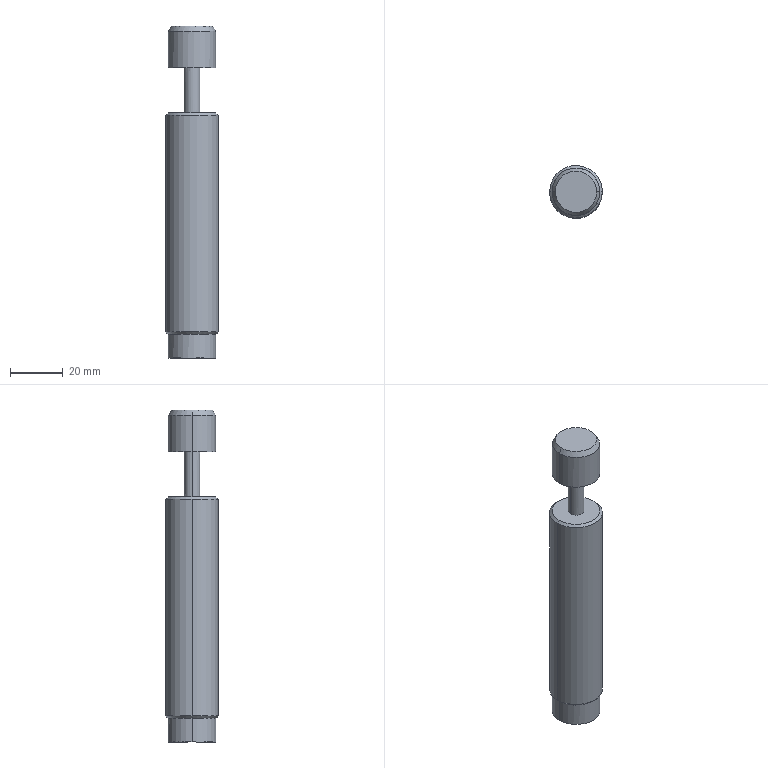Part | SolidWorks | features MoveFace 2, BaseBody 1 | 1 solid | 18 faces | box 20 x 20 x 126 mm | volume 33113 mm3 | cylinder 8 | cone 6 | plane 4 | commonest cylinder face diameters 6 x2 18 x2 18.16 x2 20 x2
STEP:
#1=CARTESIAN_POINT('',(-9.08,0.,-84.));
#2=VERTEX_POINT('',#1);
#3=CARTESIAN_POINT('',(9.08,0.,-84.));
#4=VERTEX_POINT('',#3);
#5=CARTESIAN_POINT('',(-9.08,0.,-84.));
#6=CARTESIAN_POINT('',(-9.08,1.189,-84.));
#7=CARTESIAN_POINT('',(-8.844,2.377,-84.));
#8=CARTESIAN_POINT('',(-7.934,4.573,-84.));
#9=CARTESIAN_POINT('',(-7.261,5.58,-84.));
#10=CARTESIAN_POINT('',(-5.58,7.261,-84.));
#11=CARTESIAN_POINT('',(-4.573,7.934,-84.));
#12=CARTESIAN_POINT('',(-2.377,8.844,-84.));
#13=CARTESIAN_POINT('',(-1.189,9.08,-84.));
#14=CARTESIAN_POINT('',(1.189,9.08,-84.));
#15=CARTESIAN_POINT('',(2.377,8.844,-84.));
#16=CARTESIAN_POINT('',(4.573,7.934,-84.));
#17=CARTESIAN_POINT('',(5.58,7.261,-84.));
#18=CARTESIAN_POINT('',(7.261,5.58,-84.));
#19=CARTESIAN_POINT('',(7.934,4.573,-84.));
#20=CARTESIAN_POINT('',(8.844,2.377,-84.));
#21=CARTESIAN_POINT('',(9.08,1.189,-84.));
#22=CARTESIAN_POINT('',(9.08,0.,-84.));
#23=B_SPLINE_CURVE_WITH_KNOTS('',3,(#5,#6,#7,#8,#9,#10,#11,#12,#13,#14,#15,#16,#17,#18,#19,#20,#21,#22),.UNSPECIFIED.,.F.,.F.,(4,2,2,2,2,2,2,2,4),(0.,0.3927,0.7854,1.178,1.571,1.963,2.356,2.749,3.142),.UNSPECIFIED.);
#24=EDGE_CURVE('',#2,#4,#23,.T.);
#25=ORIENTED_EDGE('',*,*,#24,.T.);
#26=CARTESIAN_POINT('',(9.08,0.,-93.));
#27=VERTEX_POINT('',#26);
#28=CARTESIAN_POINT('',(9.08,0.,-426.));
#29=DIRECTION('',(0.,0.,-1.));
#30=VECTOR('',#29,1000.);
#31=LINE('',#28,#30);
#32=EDGE_CURVE('',#4,#27,#31,.T.);
#33=ORIENTED_EDGE('',*,*,#32,.T.);
#34=CARTESIAN_POINT('',(-9.08,0.,-93.));
#35=VERTEX_POINT('',#34);
#36=CARTESIAN_POINT('',(-9.08,0.,-93.));
#37=CARTESIAN_POINT('',(-9.08,0.5962,-93.));
#38=CARTESIAN_POINT('',(-9.022,1.187,-93.));
#39=CARTESIAN_POINT('',(-8.789,2.356,-93.));
#40=CARTESIAN_POINT('',(-8.617,2.924,-93.));
#41=CARTESIAN_POINT('',(-8.161,4.026,-93.));
#42=CARTESIAN_POINT('',(-7.881,4.549,-93.));
#43=CARTESIAN_POINT('',(-7.219,5.54,-93.));
#44=CARTESIAN_POINT('',(-6.842,5.999,-93.));
#45=CARTESIAN_POINT('',(-5.999,6.842,-93.));
#46=CARTESIAN_POINT('',(-5.54,7.219,-93.));
#47=CARTESIAN_POINT('',(-4.549,7.881,-93.));
#48=CARTESIAN_POINT('',(-4.026,8.161,-93.));
#49=CARTESIAN_POINT('',(-2.924,8.617,-93.));
#50=CARTESIAN_POINT('',(-2.356,8.789,-93.));
#51=CARTESIAN_POINT('',(-1.187,9.022,-93.));
#52=CARTESIAN_POINT('',(-0.5962,9.08,-93.));
#53=CARTESIAN_POINT('',(0.5962,9.08,-93.));
#54=CARTESIAN_POINT('',(1.187,9.022,-93.));
#55=CARTESIAN_POINT('',(2.356,8.789,-93.));
#56=CARTESIAN_POINT('',(2.924,8.617,-93.));
#57=CARTESIAN_POINT('',(4.026,8.161,-93.));
#58=CARTESIAN_POINT('',(4.549,7.881,-93.));
#59=CARTESIAN_POINT('',(5.54,7.219,-93.));
#60=CARTESIAN_POINT('',(5.999,6.842,-93.));
#61=CARTESIAN_POINT('',(6.842,5.999,-93.));
#62=CARTESIAN_POINT('',(7.219,5.54,-93.));
#63=CARTESIAN_POINT('',(7.881,4.549,-93.));
#64=CARTESIAN_POINT('',(8.161,4.026,-93.));
#65=CARTESIAN_POINT('',(8.617,2.924,-93.));
#66=CARTESIAN_POINT('',(8.789,2.356,-93.));
#67=CARTESIAN_POINT('',(9.022,1.187,-93.));
#68=CARTESIAN_POINT('',(9.08,0.5962,-93.));
#69=CARTESIAN_POINT('',(9.08,0.,-93.));
#70=B_SPLINE_CURVE_WITH_KNOTS('',3,(#36,#37,#38,#39,#40,#41,#42,#43,#44,#45,#46,#47,#48,#49,#50,#51,#52,#53,#54,#55,#56,#57,#58,#59,#60,#61,#62,#63,#64,#65,#66,#67,#68,#69),.UNSPECIFIED.,.F.,.F.,(4,2,2,2,2,2,2,2,2,2,2,2,2,2,2,2,4),(0.,0.1963,0.3927,0.589,0.7854,0.9817,1.178,1.374,1.571,1.767,1.963,2.16,2.356,2.553,2.749,2.945,3.142),.UNSPECIFIED.);
#71=EDGE_CURVE('',#35,#27,#70,.T.);
#72=ORIENTED_EDGE('',*,*,#71,.F.);
#73=CARTESIAN_POINT('',(-9.08,0.,-426.));
#74=DIRECTION('',(0.,0.,-1.));
#75=VECTOR('',#74,1000.);
#76=LINE('',#73,#75);
#77=EDGE_CURVE('',#2,#35,#76,.T.);
#78=ORIENTED_EDGE('',*,*,#77,.F.);
#79=EDGE_LOOP('',(#25,#33,#72,#78));
#80=FACE_OUTER_BOUND('',#79,.T.);
#81=CARTESIAN_POINT('',(0.,0.,-426.));
#82=DIRECTION('',(0.,0.,-1.));
#83=DIRECTION('',(-1.,0.,0.));
#84=AXIS2_PLACEMENT_3D('',#81,#82,#83);
#85=CYLINDRICAL_SURFACE('',#84,9.08);
#86=ADVANCED_FACE('',(#80),#85,.T.);
#87=ORIENTED_EDGE('',*,*,#24,.F.);
#88=CARTESIAN_POINT('',(-10.,0.,-83.08));
#89=VERTEX_POINT('',#88);
#90=CARTESIAN_POINT('',(-10.,0.,-83.08));
#91=DIRECTION('',(-0.7071,0.,0.7071));
#92=VECTOR('',#91,1000.);
#93=LINE('',#90,#92);
#94=EDGE_CURVE('',#2,#89,#93,.T.);
#95=ORIENTED_EDGE('',*,*,#94,.T.);
#96=CARTESIAN_POINT('',(10.,0.,-83.08));
#97=VERTEX_POINT('',#96);
#98=CARTESIAN_POINT('',(-10.,0.,-83.08));
#99=CARTESIAN_POINT('',(-10.,1.309,-83.08));
#100=CARTESIAN_POINT('',(-9.74,2.617,-83.08));
#101=CARTESIAN_POINT('',(-8.738,5.036,-83.08));
#102=CARTESIAN_POINT('',(-7.997,6.145,-83.08));
#103=CARTESIAN_POINT('',(-6.145,7.997,-83.08));
#104=CARTESIAN_POINT('',(-5.036,8.738,-83.08));
#105=CARTESIAN_POINT('',(-2.617,9.74,-83.08));
#106=CARTESIAN_POINT('',(-1.309,10.,-83.08));
#107=CARTESIAN_POINT('',(1.309,10.,-83.08));
#108=CARTESIAN_POINT('',(2.617,9.74,-83.08));
#109=CARTESIAN_POINT('',(5.036,8.738,-83.08));
#110=CARTESIAN_POINT('',(6.145,7.997,-83.08));
#111=CARTESIAN_POINT('',(7.997,6.145,-83.08));
#112=CARTESIAN_POINT('',(8.738,5.036,-83.08));
#113=CARTESIAN_POINT('',(9.74,2.617,-83.08));
#114=CARTESIAN_POINT('',(10.,1.309,-83.08));
#115=CARTESIAN_POINT('',(10.,0.,-83.08));
#116=B_SPLINE_CURVE_WITH_KNOTS('',3,(#98,#99,#100,#101,#102,#103,#104,#105,#106,#107,#108,#109,#110,#111,#112,#113,#114,#115),.UNSPECIFIED.,.F.,.F.,(4,2,2,2,2,2,2,2,4),(0.,0.0625,0.125,0.1875,0.25,0.3125,0.375,0.4375,0.5),.UNSPECIFIED.);
#117=EDGE_CURVE('',#89,#97,#116,.T.);
#118=ORIENTED_EDGE('',*,*,#117,.T.);
#119=CARTESIAN_POINT('',(10.,0.,-83.08));
#120=DIRECTION('',(0.7071,0.,0.7071));
#121=VECTOR('',#120,1000.);
#122=LINE('',#119,#121);
#123=EDGE_CURVE('',#4,#97,#122,.T.);
#124=ORIENTED_EDGE('',*,*,#123,.F.);
#125=EDGE_LOOP('',(#87,#95,#118,#124));
#126=FACE_OUTER_BOUND('',#125,.T.);
#127=CARTESIAN_POINT('',(0.,0.,-83.08));
#128=DIRECTION('',(0.,0.,1.));
#129=DIRECTION('',(1.,0.,0.));
#130=AXIS2_PLACEMENT_3D('',#127,#128,#129);
#131=CONICAL_SURFACE('',#130,10.,0.7854);
#132=ADVANCED_FACE('',(#126),#131,.T.);
#133=CARTESIAN_POINT('',(-10.,0.,-0.92));
#134=VERTEX_POINT('',#133);
#135=CARTESIAN_POINT('',(10.,0.,-0.92));
#136=VERTEX_POINT('',#135);
#137=CARTESIAN_POINT('',(-10.,0.,-0.92));
#138=CARTESIAN_POINT('',(-10.,1.309,-0.92));
#139=CARTESIAN_POINT('',(-9.74,2.617,-0.92));
#140=CARTESIAN_POINT('',(-8.738,5.036,-0.92));
#141=CARTESIAN_POINT('',(-7.997,6.145,-0.92));
#142=CARTESIAN_POINT('',(-6.145,7.997,-0.92));
#143=CARTESIAN_POINT('',(-5.036,8.738,-0.92));
#144=CARTESIAN_POINT('',(-2.617,9.74,-0.92));
#145=CARTESIAN_POINT('',(-1.309,10.,-0.92));
#146=CARTESIAN_POINT('',(1.309,10.,-0.92));
#147=CARTESIAN_POINT('',(2.617,9.74,-0.92));
#148=CARTESIAN_POINT('',(5.036,8.738,-0.92));
#149=CARTESIAN_POINT('',(6.145,7.997,-0.92));
#150=CARTESIAN_POINT('',(7.997,6.145,-0.92));
#151=CARTESIAN_POINT('',(8.738,5.036,-0.92));
#152=CARTESIAN_POINT('',(9.74,2.617,-0.92));
#153=CARTESIAN_POINT('',(10.,1.309,-0.92));
#154=CARTESIAN_POINT('',(10.,0.,-0.92));
#155=B_SPLINE_CURVE_WITH_KNOTS('',3,(#137,#138,#139,#140,#141,#142,#143,#144,#145,#146,#147,#148,#149,#150,#151,#152,#153,#154),.UNSPECIFIED.,.F.,.F.,(4,2,2,2,2,2,2,2,4),(0.,0.3927,0.7854,1.178,1.571,1.963,2.356,2.749,3.142),.UNSPECIFIED.);
#156=EDGE_CURVE('',#134,#136,#155,.T.);
#157=ORIENTED_EDGE('',*,*,#156,.T.);
#158=CARTESIAN_POINT('',(10.,0.,-500.));
#159=DIRECTION('',(0.,0.,-1.));
#160=VECTOR('',#159,1000.);
#161=LINE('',#158,#160);
#162=EDGE_CURVE('',#136,#97,#161,.T.);
#163=ORIENTED_EDGE('',*,*,#162,.T.);
#164=ORIENTED_EDGE('',*,*,#117,.F.);
#165=CARTESIAN_POINT('',(-10.,0.,-500.));
#166=DIRECTION('',(0.,0.,-1.));
#167=VECTOR('',#166,1000.);
#168=LINE('',#165,#167);
#169=EDGE_CURVE('',#134,#89,#168,.T.);
#170=ORIENTED_EDGE('',*,*,#169,.F.);
#171=EDGE_LOOP('',(#157,#163,#164,#170));
#172=FACE_OUTER_BOUND('',#171,.T.);
#173=CARTESIAN_POINT('',(0.,0.,-500.));
#174=DIRECTION('',(0.,0.,-1.));
#175=DIRECTION('',(-1.,0.,0.));
#176=AXIS2_PLACEMENT_3D('',#173,#174,#175);
#177=CYLINDRICAL_SURFACE('',#176,10.);
#178=ADVANCED_FACE('',(#172),#177,.T.);
#179=CARTESIAN_POINT('',(-9.08,0.,0.));
#180=VERTEX_POINT('',#179);
#181=CARTESIAN_POINT('',(9.08,0.,0.));
#182=VERTEX_POINT('',#181);
#183=CARTESIAN_POINT('',(-9.08,0.,0.));
#184=CARTESIAN_POINT('',(-9.08,1.189,0.));
#185=CARTESIAN_POINT('',(-8.844,2.377,0.));
#186=CARTESIAN_POINT('',(-7.934,4.573,0.));
#187=CARTESIAN_POINT('',(-7.261,5.58,0.));
#188=CARTESIAN_POINT('',(-5.58,7.261,0.));
#189=CARTESIAN_POINT('',(-4.573,7.934,0.));
#190=CARTESIAN_POINT('',(-2.377,8.844,0.));
#191=CARTESIAN_POINT('',(-1.189,9.08,0.));
#192=CARTESIAN_POINT('',(1.189,9.08,0.));
#193=CARTESIAN_POINT('',(2.377,8.844,0.));
#194=CARTESIAN_POINT('',(4.573,7.934,0.));
#195=CARTESIAN_POINT('',(5.58,7.261,0.));
#196=CARTESIAN_POINT('',(7.261,5.58,0.));
#197=CARTESIAN_POINT('',(7.934,4.573,0.));
#198=CARTESIAN_POINT('',(8.844,2.377,0.));
#199=CARTESIAN_POINT('',(9.08,1.189,0.));
#200=CARTESIAN_POINT('',(9.08,0.,0.));
#201=B_SPLINE_CURVE_WITH_KNOTS('',3,(#183,#184,#185,#186,#187,#188,#189,#190,#191,#192,#193,#194,#195,#196,#197,#198,#199,#200),.UNSPECIFIED.,.F.,.F.,(4,2,2,2,2,2,2,2,4),(0.,0.3927,0.7854,1.178,1.571,1.963,2.356,2.749,3.142),.UNSPECIFIED.);
#202=EDGE_CURVE('',#180,#182,#201,.T.);
#203=ORIENTED_EDGE('',*,*,#202,.T.);
#204=CARTESIAN_POINT('',(9.08,0.,0.));
#205=DIRECTION('',(0.7071,0.,-0.7071));
#206=VECTOR('',#205,1000.);
#207=LINE('',#204,#206);
#208=EDGE_CURVE('',#182,#136,#207,.T.);
#209=ORIENTED_EDGE('',*,*,#208,.T.);
#210=ORIENTED_EDGE('',*,*,#156,.F.);
#211=CARTESIAN_POINT('',(-9.08,0.,0.));
#212=DIRECTION('',(-0.7071,0.,-0.7071));
#213=VECTOR('',#212,1000.);
#214=LINE('',#211,#213);
#215=EDGE_CURVE('',#180,#134,#214,.T.);
#216=ORIENTED_EDGE('',*,*,#215,.F.);
#217=EDGE_LOOP('',(#203,#209,#210,#216));
#218=FACE_OUTER_BOUND('',#217,.T.);
#219=CARTESIAN_POINT('',(0.,0.,0.));
#220=DIRECTION('',(0.,0.,-1.));
#221=DIRECTION('',(-1.,0.,0.));
#222=AXIS2_PLACEMENT_3D('',#219,#220,#221);
#223=CONICAL_SURFACE('',#222,9.08,0.7854);
#224=ADVANCED_FACE('',(#218),#223,.T.);
#225=CARTESIAN_POINT('',(-3.,0.,17.2));
#226=VERTEX_POINT('',#225);
#227=CARTESIAN_POINT('',(3.,0.,17.2));
#228=VERTEX_POINT('',#227);
#229=CARTESIAN_POINT('',(-3.,0.,17.2));
#230=CARTESIAN_POINT('',(-3.,0.3927,17.2));
#231=CARTESIAN_POINT('',(-2.922,0.7852,17.2));
#232=CARTESIAN_POINT('',(-2.621,1.511,17.2));
#233=CARTESIAN_POINT('',(-2.399,1.844,17.2));
#234=CARTESIAN_POINT('',(-1.844,2.399,17.2));
#235=CARTESIAN_POINT('',(-1.511,2.621,17.2));
#236=CARTESIAN_POINT('',(-0.7852,2.922,17.2));
#237=CARTESIAN_POINT('',(-0.3927,3.,17.2));
#238=CARTESIAN_POINT('',(0.3927,3.,17.2));
#239=CARTESIAN_POINT('',(0.7852,2.922,17.2));
#240=CARTESIAN_POINT('',(1.511,2.621,17.2));
#241=CARTESIAN_POINT('',(1.844,2.399,17.2));
#242=CARTESIAN_POINT('',(2.399,1.844,17.2));
#243=CARTESIAN_POINT('',(2.621,1.511,17.2));
#244=CARTESIAN_POINT('',(2.922,0.7852,17.2));
#245=CARTESIAN_POINT('',(3.,0.3927,17.2));
#246=CARTESIAN_POINT('',(3.,0.,17.2));
#247=B_SPLINE_CURVE_WITH_KNOTS('',3,(#229,#230,#231,#232,#233,#234,#235,#236,#237,#238,#239,#240,#241,#242,#243,#244,#245,#246),.UNSPECIFIED.,.F.,.F.,(4,2,2,2,2,2,2,2,4),(0.,0.3927,0.7854,1.178,1.571,1.963,2.356,2.749,3.142),.UNSPECIFIED.);
#248=EDGE_CURVE('',#226,#228,#247,.T.);
#249=ORIENTED_EDGE('',*,*,#248,.T.);
#250=CARTESIAN_POINT('',(3.,0.,0.));
#251=VERTEX_POINT('',#250);
#252=CARTESIAN_POINT('',(3.,0.,-532.8));
#253=DIRECTION('',(0.,0.,-1.));
#254=VECTOR('',#253,1000.);
#255=LINE('',#252,#254);
#256=EDGE_CURVE('',#228,#251,#255,.T.);
#257=ORIENTED_EDGE('',*,*,#256,.T.);
#258=CARTESIAN_POINT('',(-3.,0.,0.));
#259=VERTEX_POINT('',#258);
#260=CARTESIAN_POINT('',(0.,0.,0.));
#261=DIRECTION('',(0.,0.,-1.));
#262=DIRECTION('',(-1.,0.,0.));
#263=AXIS2_PLACEMENT_3D('',#260,#261,#262);
#264=CIRCLE('',#263,3.);
#265=EDGE_CURVE('',#259,#251,#264,.T.);
#266=ORIENTED_EDGE('',*,*,#265,.F.);
#267=CARTESIAN_POINT('',(-3.,0.,-532.8));
#268=DIRECTION('',(0.,0.,-1.));
#269=VECTOR('',#268,1000.);
#270=LINE('',#267,#269);
#271=EDGE_CURVE('',#226,#259,#270,.T.);
#272=ORIENTED_EDGE('',*,*,#271,.F.);
#273=EDGE_LOOP('',(#249,#257,#266,#272));
#274=FACE_OUTER_BOUND('',#273,.T.);
#275=CARTESIAN_POINT('',(0.,0.,-532.8));
#276=DIRECTION('',(0.,0.,-1.));
#277=DIRECTION('',(-1.,0.,0.));
#278=AXIS2_PLACEMENT_3D('',#275,#276,#277);
#279=CYLINDRICAL_SURFACE('',#278,3.);
#280=ADVANCED_FACE('',(#274),#279,.T.);
#281=CARTESIAN_POINT('',(-9.,0.,31.));
#282=VERTEX_POINT('',#281);
#283=CARTESIAN_POINT('',(9.,0.,31.));
#284=VERTEX_POINT('',#283);
#285=CARTESIAN_POINT('',(-9.,0.,31.));
#286=CARTESIAN_POINT('',(-9.,1.178,31.));
#287=CARTESIAN_POINT('',(-8.766,2.356,31.));
#288=CARTESIAN_POINT('',(-7.864,4.533,31.));
#289=CARTESIAN_POINT('',(-7.197,5.531,31.));
#290=CARTESIAN_POINT('',(-5.531,7.197,31.));
#291=CARTESIAN_POINT('',(-4.533,7.864,31.));
#292=CARTESIAN_POINT('',(-2.356,8.766,31.));
#293=CARTESIAN_POINT('',(-1.178,9.,31.));
#294=CARTESIAN_POINT('',(1.178,9.,31.));
#295=CARTESIAN_POINT('',(2.356,8.766,31.));
#296=CARTESIAN_POINT('',(4.533,7.864,31.));
#297=CARTESIAN_POINT('',(5.531,7.197,31.));
#298=CARTESIAN_POINT('',(7.197,5.531,31.));
#299=CARTESIAN_POINT('',(7.864,4.533,31.));
#300=CARTESIAN_POINT('',(8.766,2.356,31.));
#301=CARTESIAN_POINT('',(9.,1.178,31.));
#302=CARTESIAN_POINT('',(9.,0.,31.));
#303=B_SPLINE_CURVE_WITH_KNOTS('',3,(#285,#286,#287,#288,#289,#290,#291,#292,#293,#294,#295,#296,#297,#298,#299,#300,#301,#302),.UNSPECIFIED.,.F.,.F.,(4,2,2,2,2,2,2,2,4),(0.,0.3927,0.7854,1.178,1.571,1.963,2.356,2.749,3.142),.UNSPECIFIED.);
#304=EDGE_CURVE('',#282,#284,#303,.T.);
#305=ORIENTED_EDGE('',*,*,#304,.T.);
#306=CARTESIAN_POINT('',(9.,0.,17.2));
#307=VERTEX_POINT('',#306);
#308=CARTESIAN_POINT('',(9.,0.,-532.8));
#309=DIRECTION('',(0.,0.,-1.));
#310=VECTOR('',#309,1000.);
#311=LINE('',#308,#310);
#312=EDGE_CURVE('',#284,#307,#311,.T.);
#313=ORIENTED_EDGE('',*,*,#312,.T.);
#314=CARTESIAN_POINT('',(-9.,0.,17.2));
#315=VERTEX_POINT('',#314);
#316=CARTESIAN_POINT('',(-9.,0.,17.2));
#317=CARTESIAN_POINT('',(-9.,0.5909,17.2));
#318=CARTESIAN_POINT('',(-8.942,1.176,17.2));
#319=CARTESIAN_POINT('',(-8.712,2.335,17.2));
#320=CARTESIAN_POINT('',(-8.541,2.898,17.2));
#321=CARTESIAN_POINT('',(-8.089,3.99,17.2));
#322=CARTESIAN_POINT('',(-7.812,4.509,17.2));
#323=CARTESIAN_POINT('',(-7.155,5.491,17.2));
#324=CARTESIAN_POINT('',(-6.782,5.946,17.2));
#325=CARTESIAN_POINT('',(-5.946,6.782,17.2));
#326=CARTESIAN_POINT('',(-5.491,7.155,17.2));
#327=CARTESIAN_POINT('',(-4.509,7.812,17.2));
#328=CARTESIAN_POINT('',(-3.99,8.089,17.2));
#329=CARTESIAN_POINT('',(-2.898,8.541,17.2));
#330=CARTESIAN_POINT('',(-2.335,8.712,17.2));
#331=CARTESIAN_POINT('',(-1.176,8.942,17.2));
#332=CARTESIAN_POINT('',(-0.5909,9.,17.2));
#333=CARTESIAN_POINT('',(0.5909,9.,17.2));
#334=CARTESIAN_POINT('',(1.176,8.942,17.2));
#335=CARTESIAN_POINT('',(2.335,8.712,17.2));
#336=CARTESIAN_POINT('',(2.898,8.541,17.2));
#337=CARTESIAN_POINT('',(3.99,8.089,17.2));
#338=CARTESIAN_POINT('',(4.509,7.812,17.2));
#339=CARTESIAN_POINT('',(5.491,7.155,17.2));
#340=CARTESIAN_POINT('',(5.946,6.782,17.2));
#341=CARTESIAN_POINT('',(6.782,5.946,17.2));
#342=CARTESIAN_POINT('',(7.155,5.491,17.2));
#343=CARTESIAN_POINT('',(7.812,4.509,17.2));
#344=CARTESIAN_POINT('',(8.089,3.99,17.2));
#345=CARTESIAN_POINT('',(8.541,2.898,17.2));
#346=CARTESIAN_POINT('',(8.712,2.335,17.2));
#347=CARTESIAN_POINT('',(8.942,1.176,17.2));
#348=CARTESIAN_POINT('',(9.,0.5909,17.2));
#349=CARTESIAN_POINT('',(9.,0.,17.2));
#350=B_SPLINE_CURVE_WITH_KNOTS('',3,(#316,#317,#318,#319,#320,#321,#322,#323,#324,#325,#326,#327,#328,#329,#330,#331,#332,#333,#334,#335,#336,#337,#338,#339,#340,#341,#342,#343,#344,#345,#346,#347,#348,#349),.UNSPECIFIED.,.F.,.F.,(4,2,2,2,2,2,2,2,2,2,2,2,2,2,2,2,4),(0.,0.1963,0.3927,0.589,0.7854,0.9817,1.178,1.374,1.571,1.767,1.963,2.16,2.356,2.553,2.749,2.945,3.142),.UNSPECIFIED.);
#351=EDGE_CURVE('',#315,#307,#350,.T.);
#352=ORIENTED_EDGE('',*,*,#351,.F.);
#353=CARTESIAN_POINT('',(-9.,0.,-532.8));
#354=DIRECTION('',(0.,0.,-1.));
#355=VECTOR('',#354,1000.);
#356=LINE('',#353,#355);
#357=EDGE_CURVE('',#282,#315,#356,.T.);
#358=ORIENTED_EDGE('',*,*,#357,.F.);
#359=EDGE_LOOP('',(#305,#313,#352,#358));
#360=FACE_OUTER_BOUND('',#359,.T.);
#361=CARTESIAN_POINT('',(0.,0.,-532.8));
#362=DIRECTION('',(0.,0.,-1.));
#363=DIRECTION('',(-1.,0.,0.));
#364=AXIS2_PLACEMENT_3D('',#361,#362,#363);
#365=CYLINDRICAL_SURFACE('',#364,9.);
#366=ADVANCED_FACE('',(#360),#365,.T.);
#367=CARTESIAN_POINT('',(-7.845,0.,33.));
#368=VERTEX_POINT('',#367);
#369=CARTESIAN_POINT('',(7.845,0.,33.));
#370=VERTEX_POINT('',#369);
#371=CARTESIAN_POINT('',(-7.845,0.,33.));
#372=CARTESIAN_POINT('',(-7.845,1.027,33.));
#373=CARTESIAN_POINT('',(-7.641,2.053,33.));
#374=CARTESIAN_POINT('',(-6.855,3.951,33.));
#375=CARTESIAN_POINT('',(-6.274,4.821,33.));
#376=CARTESIAN_POINT('',(-4.821,6.274,33.));
#377=CARTESIAN_POINT('',(-3.951,6.855,33.));
#378=CARTESIAN_POINT('',(-2.053,7.641,33.));
#379=CARTESIAN_POINT('',(-1.027,7.845,33.));
#380=CARTESIAN_POINT('',(1.027,7.845,33.));
#381=CARTESIAN_POINT('',(2.053,7.641,33.));
#382=CARTESIAN_POINT('',(3.951,6.855,33.));
#383=CARTESIAN_POINT('',(4.821,6.274,33.));
#384=CARTESIAN_POINT('',(6.274,4.821,33.));
#385=CARTESIAN_POINT('',(6.855,3.951,33.));
#386=CARTESIAN_POINT('',(7.641,2.053,33.));
#387=CARTESIAN_POINT('',(7.845,1.027,33.));
#388=CARTESIAN_POINT('',(7.845,0.,33.));
#389=B_SPLINE_CURVE_WITH_KNOTS('',3,(#371,#372,#373,#374,#375,#376,#377,#378,#379,#380,#381,#382,#383,#384,#385,#386,#387,#388),.UNSPECIFIED.,.F.,.F.,(4,2,2,2,2,2,2,2,4),(0.,0.3927,0.7854,1.178,1.571,1.963,2.356,2.749,3.142),.UNSPECIFIED.);
#390=EDGE_CURVE('',#368,#370,#389,.T.);
#391=ORIENTED_EDGE('',*,*,#390,.T.);
#392=CARTESIAN_POINT('',(7.845,0.,33.));
#393=DIRECTION('',(0.5,0.,-0.866));
#394=VECTOR('',#393,1000.);
#395=LINE('',#392,#394);
#396=EDGE_CURVE('',#370,#284,#395,.T.);
#397=ORIENTED_EDGE('',*,*,#396,.T.);
#398=ORIENTED_EDGE('',*,*,#304,.F.);
#399=CARTESIAN_POINT('',(-7.845,0.,33.));
#400=DIRECTION('',(-0.5,0.,-0.866));
#401=VECTOR('',#400,1000.);
#402=LINE('',#399,#401);
#403=EDGE_CURVE('',#368,#282,#402,.T.);
#404=ORIENTED_EDGE('',*,*,#403,.F.);
#405=EDGE_LOOP('',(#391,#397,#398,#404));
#406=FACE_OUTER_BOUND('',#405,.T.);
#407=CARTESIAN_POINT('',(0.,0.,33.));
#408=DIRECTION('',(0.,0.,-1.));
#409=DIRECTION('',(-1.,0.,0.));
#410=AXIS2_PLACEMENT_3D('',#407,#408,#409);
#411=CONICAL_SURFACE('',#410,7.845,0.5236);
#412=ADVANCED_FACE('',(#406),#411,.T.);
#413=ORIENTED_EDGE('',*,*,#390,.F.);
#414=CARTESIAN_POINT('',(7.845,0.,33.));
#415=CARTESIAN_POINT('',(7.845,-1.027,33.));
#416=CARTESIAN_POINT('',(7.641,-2.053,33.));
#417=CARTESIAN_POINT('',(6.855,-3.951,33.));
#418=CARTESIAN_POINT('',(6.274,-4.821,33.));
#419=CARTESIAN_POINT('',(4.821,-6.274,33.));
#420=CARTESIAN_POINT('',(3.951,-6.855,33.));
#421=CARTESIAN_POINT('',(2.053,-7.641,33.));
#422=CARTESIAN_POINT('',(1.027,-7.845,33.));
#423=CARTESIAN_POINT('',(-1.027,-7.845,33.));
#424=CARTESIAN_POINT('',(-2.053,-7.641,33.));
#425=CARTESIAN_POINT('',(-3.951,-6.855,33.));
#426=CARTESIAN_POINT('',(-4.821,-6.274,33.));
#427=CARTESIAN_POINT('',(-6.274,-4.821,33.));
#428=CARTESIAN_POINT('',(-6.855,-3.951,33.));
#429=CARTESIAN_POINT('',(-7.641,-2.053,33.));
#430=CARTESIAN_POINT('',(-7.845,-1.027,33.));
#431=CARTESIAN_POINT('',(-7.845,0.,33.));
#432=B_SPLINE_CURVE_WITH_KNOTS('',3,(#414,#415,#416,#417,#418,#419,#420,#421,#422,#423,#424,#425,#426,#427,#428,#429,#430,#431),.UNSPECIFIED.,.F.,.F.,(4,2,2,2,2,2,2,2,4),(3.142,3.534,3.927,4.32,4.712,5.105,5.498,5.89,6.283),.UNSPECIFIED.);
#433=EDGE_CURVE('',#370,#368,#432,.T.);
#434=ORIENTED_EDGE('',*,*,#433,.F.);
#435=EDGE_LOOP('',(#413,#434));
#436=FACE_OUTER_BOUND('',#435,.T.);
#437=CARTESIAN_POINT('',(0.,0.,33.));
#438=DIRECTION('',(0.,0.,-1.));
#439=DIRECTION('',(-1.,0.,0.));
#440=AXIS2_PLACEMENT_3D('',#437,#438,#439);
#441=PLANE('',#440);
#442=ADVANCED_FACE('',(#436),#441,.F.);
#443=ORIENTED_EDGE('',*,*,#396,.F.);
#444=ORIENTED_EDGE('',*,*,#433,.T.);
#445=ORIENTED_EDGE('',*,*,#403,.T.);
#446=CARTESIAN_POINT('',(9.,0.,31.));
#447=CARTESIAN_POINT('',(9.,-1.178,31.));
#448=CARTESIAN_POINT('',(8.766,-2.356,31.));
#449=CARTESIAN_POINT('',(7.864,-4.533,31.));
#450=CARTESIAN_POINT('',(7.197,-5.531,31.));
#451=CARTESIAN_POINT('',(5.531,-7.197,31.));
#452=CARTESIAN_POINT('',(4.533,-7.864,31.));
#453=CARTESIAN_POINT('',(2.356,-8.766,31.));
#454=CARTESIAN_POINT('',(1.178,-9.,31.));
#455=CARTESIAN_POINT('',(-1.178,-9.,31.));
#456=CARTESIAN_POINT('',(-2.356,-8.766,31.));
#457=CARTESIAN_POINT('',(-4.533,-7.864,31.));
#458=CARTESIAN_POINT('',(-5.531,-7.197,31.));
#459=CARTESIAN_POINT('',(-7.197,-5.531,31.));
#460=CARTESIAN_POINT('',(-7.864,-4.533,31.));
#461=CARTESIAN_POINT('',(-8.766,-2.356,31.));
#462=CARTESIAN_POINT('',(-9.,-1.178,31.));
#463=CARTESIAN_POINT('',(-9.,0.,31.));
#464=B_SPLINE_CURVE_WITH_KNOTS('',3,(#446,#447,#448,#449,#450,#451,#452,#453,#454,#455,#456,#457,#458,#459,#460,#461,#462,#463),.UNSPECIFIED.,.F.,.F.,(4,2,2,2,2,2,2,2,4),(3.142,3.534,3.927,4.32,4.712,5.105,5.498,5.89,6.283),.UNSPECIFIED.);
#465=EDGE_CURVE('',#284,#282,#464,.T.);
#466=ORIENTED_EDGE('',*,*,#465,.F.);
#467=EDGE_LOOP('',(#443,#444,#445,#466));
#468=FACE_OUTER_BOUND('',#467,.T.);
#469=CARTESIAN_POINT('',(0.,0.,33.));
#470=DIRECTION('',(0.,0.,-1.));
#471=DIRECTION('',(-1.,0.,0.));
#472=AXIS2_PLACEMENT_3D('',#469,#470,#471);
#473=CONICAL_SURFACE('',#472,7.845,0.5236);
#474=ADVANCED_FACE('',(#468),#473,.T.);
#475=ORIENTED_EDGE('',*,*,#312,.F.);
#476=ORIENTED_EDGE('',*,*,#465,.T.);
#477=ORIENTED_EDGE('',*,*,#357,.T.);
#478=CARTESIAN_POINT('',(9.,0.,17.2));
#479=CARTESIAN_POINT('',(9.,-0.5909,17.2));
#480=CARTESIAN_POINT('',(8.942,-1.176,17.2));
#481=CARTESIAN_POINT('',(8.712,-2.335,17.2));
#482=CARTESIAN_POINT('',(8.541,-2.898,17.2));
#483=CARTESIAN_POINT('',(8.089,-3.99,17.2));
#484=CARTESIAN_POINT('',(7.812,-4.509,17.2));
#485=CARTESIAN_POINT('',(7.155,-5.491,17.2));
#486=CARTESIAN_POINT('',(6.782,-5.946,17.2));
#487=CARTESIAN_POINT('',(5.946,-6.782,17.2));
#488=CARTESIAN_POINT('',(5.491,-7.155,17.2));
#489=CARTESIAN_POINT('',(4.509,-7.812,17.2));
#490=CARTESIAN_POINT('',(3.99,-8.089,17.2));
#491=CARTESIAN_POINT('',(2.898,-8.541,17.2));
#492=CARTESIAN_POINT('',(2.335,-8.712,17.2));
#493=CARTESIAN_POINT('',(1.176,-8.942,17.2));
#494=CARTESIAN_POINT('',(0.5909,-9.,17.2));
#495=CARTESIAN_POINT('',(-0.5909,-9.,17.2));
#496=CARTESIAN_POINT('',(-1.176,-8.942,17.2));
#497=CARTESIAN_POINT('',(-2.335,-8.712,17.2));
#498=CARTESIAN_POINT('',(-2.898,-8.541,17.2));
#499=CARTESIAN_POINT('',(-3.99,-8.089,17.2));
#500=CARTESIAN_POINT('',(-4.509,-7.812,17.2));
#501=CARTESIAN_POINT('',(-5.491,-7.155,17.2));
#502=CARTESIAN_POINT('',(-5.946,-6.782,17.2));
#503=CARTESIAN_POINT('',(-6.782,-5.946,17.2));
#504=CARTESIAN_POINT('',(-7.155,-5.491,17.2));
#505=CARTESIAN_POINT('',(-7.812,-4.509,17.2));
#506=CARTESIAN_POINT('',(-8.089,-3.99,17.2));
#507=CARTESIAN_POINT('',(-8.541,-2.898,17.2));
#508=CARTESIAN_POINT('',(-8.712,-2.335,17.2));
#509=CARTESIAN_POINT('',(-8.942,-1.176,17.2));
#510=CARTESIAN_POINT('',(-9.,-0.5909,17.2));
#511=CARTESIAN_POINT('',(-9.,0.,17.2));
#512=B_SPLINE_CURVE_WITH_KNOTS('',3,(#478,#479,#480,#481,#482,#483,#484,#485,#486,#487,#488,#489,#490,#491,#492,#493,#494,#495,#496,#497,#498,#499,#500,#501,#502,#503,#504,#505,#506,#507,#508,#509,#510,#511),.UNSPECIFIED.,.F.,.F.,(4,2,2,2,2,2,2,2,2,2,2,2,2,2,2,2,4),(3.142,3.338,3.534,3.731,3.927,4.123,4.32,4.516,4.712,4.909,5.105,5.301,5.498,5.694,5.89,6.087,6.283),.UNSPECIFIED.);
#513=EDGE_CURVE('',#307,#315,#512,.T.);
#514=ORIENTED_EDGE('',*,*,#513,.F.);
#515=EDGE_LOOP('',(#475,#476,#477,#514));
#516=FACE_OUTER_BOUND('',#515,.T.);
#517=CARTESIAN_POINT('',(0.,0.,-532.8));
#518=DIRECTION('',(0.,0.,-1.));
#519=DIRECTION('',(-1.,0.,0.));
#520=AXIS2_PLACEMENT_3D('',#517,#518,#519);
#521=CYLINDRICAL_SURFACE('',#520,9.);
#522=ADVANCED_FACE('',(#516),#521,.T.);
#523=ORIENTED_EDGE('',*,*,#248,.F.);
#524=CARTESIAN_POINT('',(3.,0.,17.2));
#525=CARTESIAN_POINT('',(3.,-0.3927,17.2));
#526=CARTESIAN_POINT('',(2.922,-0.7852,17.2));
#527=CARTESIAN_POINT('',(2.621,-1.511,17.2));
#528=CARTESIAN_POINT('',(2.399,-1.844,17.2));
#529=CARTESIAN_POINT('',(1.844,-2.399,17.2));
#530=CARTESIAN_POINT('',(1.511,-2.621,17.2));
#531=CARTESIAN_POINT('',(0.7852,-2.922,17.2));
#532=CARTESIAN_POINT('',(0.3927,-3.,17.2));
#533=CARTESIAN_POINT('',(-0.3927,-3.,17.2));
#534=CARTESIAN_POINT('',(-0.7852,-2.922,17.2));
#535=CARTESIAN_POINT('',(-1.511,-2.621,17.2));
#536=CARTESIAN_POINT('',(-1.844,-2.399,17.2));
#537=CARTESIAN_POINT('',(-2.399,-1.844,17.2));
#538=CARTESIAN_POINT('',(-2.621,-1.511,17.2));
#539=CARTESIAN_POINT('',(-2.922,-0.7852,17.2));
#540=CARTESIAN_POINT('',(-3.,-0.3927,17.2));
#541=CARTESIAN_POINT('',(-3.,0.,17.2));
#542=B_SPLINE_CURVE_WITH_KNOTS('',3,(#524,#525,#526,#527,#528,#529,#530,#531,#532,#533,#534,#535,#536,#537,#538,#539,#540,#541),.UNSPECIFIED.,.F.,.F.,(4,2,2,2,2,2,2,2,4),(3.142,3.534,3.927,4.32,4.712,5.105,5.498,5.89,6.283),.UNSPECIFIED.);
#543=EDGE_CURVE('',#228,#226,#542,.T.);
#544=ORIENTED_EDGE('',*,*,#543,.F.);
#545=EDGE_LOOP('',(#523,#544));
#546=FACE_BOUND('',#545,.T.);
#547=ORIENTED_EDGE('',*,*,#351,.T.);
#548=ORIENTED_EDGE('',*,*,#513,.T.);
#549=EDGE_LOOP('',(#547,#548));
#550=FACE_OUTER_BOUND('',#549,.T.);
#551=CARTESIAN_POINT('',(0.,9.,17.2));
#552=DIRECTION('',(0.,0.,1.));
#553=DIRECTION('',(1.,0.,0.));
#554=AXIS2_PLACEMENT_3D('',#551,#552,#553);
#555=PLANE('',#554);
#556=ADVANCED_FACE('',(#546,#550),#555,.F.);
#557=ORIENTED_EDGE('',*,*,#256,.F.);
#558=ORIENTED_EDGE('',*,*,#543,.T.);
#559=ORIENTED_EDGE('',*,*,#271,.T.);
#560=CARTESIAN_POINT('',(0.,0.,0.));
#561=DIRECTION('',(0.,0.,-1.));
#562=DIRECTION('',(-1.,0.,0.));
#563=AXIS2_PLACEMENT_3D('',#560,#561,#562);
#564=CIRCLE('',#563,3.);
#565=EDGE_CURVE('',#251,#259,#564,.T.);
#566=ORIENTED_EDGE('',*,*,#565,.F.);
#567=EDGE_LOOP('',(#557,#558,#559,#566));
#568=FACE_OUTER_BOUND('',#567,.T.);
#569=CARTESIAN_POINT('',(0.,0.,-532.8));
#570=DIRECTION('',(0.,0.,-1.));
#571=DIRECTION('',(-1.,0.,0.));
#572=AXIS2_PLACEMENT_3D('',#569,#570,#571);
#573=CYLINDRICAL_SURFACE('',#572,3.);
#574=ADVANCED_FACE('',(#568),#573,.T.);
#575=ORIENTED_EDGE('',*,*,#202,.F.);
#576=CARTESIAN_POINT('',(9.08,0.,0.));
#577=CARTESIAN_POINT('',(9.08,-1.189,0.));
#578=CARTESIAN_POINT('',(8.844,-2.377,0.));
#579=CARTESIAN_POINT('',(7.934,-4.573,0.));
#580=CARTESIAN_POINT('',(7.261,-5.58,0.));
#581=CARTESIAN_POINT('',(5.58,-7.261,0.));
#582=CARTESIAN_POINT('',(4.573,-7.934,0.));
#583=CARTESIAN_POINT('',(2.377,-8.844,0.));
#584=CARTESIAN_POINT('',(1.189,-9.08,0.));
#585=CARTESIAN_POINT('',(-1.189,-9.08,0.));
#586=CARTESIAN_POINT('',(-2.377,-8.844,0.));
#587=CARTESIAN_POINT('',(-4.573,-7.934,0.));
#588=CARTESIAN_POINT('',(-5.58,-7.261,0.));
#589=CARTESIAN_POINT('',(-7.261,-5.58,0.));
#590=CARTESIAN_POINT('',(-7.934,-4.573,0.));
#591=CARTESIAN_POINT('',(-8.844,-2.377,0.));
#592=CARTESIAN_POINT('',(-9.08,-1.189,0.));
#593=CARTESIAN_POINT('',(-9.08,0.,0.));
#594=B_SPLINE_CURVE_WITH_KNOTS('',3,(#576,#577,#578,#579,#580,#581,#582,#583,#584,#585,#586,#587,#588,#589,#590,#591,#592,#593),.UNSPECIFIED.,.F.,.F.,(4,2,2,2,2,2,2,2,4),(3.142,3.534,3.927,4.32,4.712,5.105,5.498,5.89,6.283),.UNSPECIFIED.);
#595=EDGE_CURVE('',#182,#180,#594,.T.);
#596=ORIENTED_EDGE('',*,*,#595,.F.);
#597=EDGE_LOOP('',(#575,#596));
#598=FACE_OUTER_BOUND('',#597,.T.);
#599=ORIENTED_EDGE('',*,*,#265,.T.);
#600=ORIENTED_EDGE('',*,*,#565,.T.);
#601=EDGE_LOOP('',(#599,#600));
#602=FACE_BOUND('',#601,.T.);
#603=CARTESIAN_POINT('',(0.,3.,0.));
#604=DIRECTION('',(0.,0.,-1.));
#605=DIRECTION('',(-1.,0.,0.));
#606=AXIS2_PLACEMENT_3D('',#603,#604,#605);
#607=PLANE('',#606);
#608=ADVANCED_FACE('',(#598,#602),#607,.F.);
#609=ORIENTED_EDGE('',*,*,#208,.F.);
#610=ORIENTED_EDGE('',*,*,#595,.T.);
#611=ORIENTED_EDGE('',*,*,#215,.T.);
#612=CARTESIAN_POINT('',(10.,0.,-0.92));
#613=CARTESIAN_POINT('',(10.,-1.309,-0.92));
#614=CARTESIAN_POINT('',(9.74,-2.617,-0.92));
#615=CARTESIAN_POINT('',(8.738,-5.036,-0.92));
#616=CARTESIAN_POINT('',(7.997,-6.145,-0.92));
#617=CARTESIAN_POINT('',(6.145,-7.997,-0.92));
#618=CARTESIAN_POINT('',(5.036,-8.738,-0.92));
#619=CARTESIAN_POINT('',(2.617,-9.74,-0.92));
#620=CARTESIAN_POINT('',(1.309,-10.,-0.92));
#621=CARTESIAN_POINT('',(-1.309,-10.,-0.92));
#622=CARTESIAN_POINT('',(-2.617,-9.74,-0.92));
#623=CARTESIAN_POINT('',(-5.036,-8.738,-0.92));
#624=CARTESIAN_POINT('',(-6.145,-7.997,-0.92));
#625=CARTESIAN_POINT('',(-7.997,-6.145,-0.92));
#626=CARTESIAN_POINT('',(-8.738,-5.036,-0.92));
#627=CARTESIAN_POINT('',(-9.74,-2.617,-0.92));
#628=CARTESIAN_POINT('',(-10.,-1.309,-0.92));
#629=CARTESIAN_POINT('',(-10.,0.,-0.92));
#630=B_SPLINE_CURVE_WITH_KNOTS('',3,(#612,#613,#614,#615,#616,#617,#618,#619,#620,#621,#622,#623,#624,#625,#626,#627,#628,#629),.UNSPECIFIED.,.F.,.F.,(4,2,2,2,2,2,2,2,4),(3.142,3.534,3.927,4.32,4.712,5.105,5.498,5.89,6.283),.UNSPECIFIED.);
#631=EDGE_CURVE('',#136,#134,#630,.T.);
#632=ORIENTED_EDGE('',*,*,#631,.F.);
#633=EDGE_LOOP('',(#609,#610,#611,#632));
#634=FACE_OUTER_BOUND('',#633,.T.);
#635=CARTESIAN_POINT('',(0.,0.,0.));
#636=DIRECTION('',(0.,0.,-1.));
#637=DIRECTION('',(-1.,0.,0.));
#638=AXIS2_PLACEMENT_3D('',#635,#636,#637);
#639=CONICAL_SURFACE('',#638,9.08,0.7854);
#640=ADVANCED_FACE('',(#634),#639,.T.);
#641=ORIENTED_EDGE('',*,*,#162,.F.);
#642=ORIENTED_EDGE('',*,*,#631,.T.);
#643=ORIENTED_EDGE('',*,*,#169,.T.);
#644=CARTESIAN_POINT('',(10.,0.,-83.08));
#645=CARTESIAN_POINT('',(10.,-1.309,-83.08));
#646=CARTESIAN_POINT('',(9.74,-2.617,-83.08));
#647=CARTESIAN_POINT('',(8.738,-5.036,-83.08));
#648=CARTESIAN_POINT('',(7.997,-6.145,-83.08));
#649=CARTESIAN_POINT('',(6.145,-7.997,-83.08));
#650=CARTESIAN_POINT('',(5.036,-8.738,-83.08));
#651=CARTESIAN_POINT('',(2.617,-9.74,-83.08));
#652=CARTESIAN_POINT('',(1.309,-10.,-83.08));
#653=CARTESIAN_POINT('',(-1.309,-10.,-83.08));
#654=CARTESIAN_POINT('',(-2.617,-9.74,-83.08));
#655=CARTESIAN_POINT('',(-5.036,-8.738,-83.08));
#656=CARTESIAN_POINT('',(-6.145,-7.997,-83.08));
#657=CARTESIAN_POINT('',(-7.997,-6.145,-83.08));
#658=CARTESIAN_POINT('',(-8.738,-5.036,-83.08));
#659=CARTESIAN_POINT('',(-9.74,-2.617,-83.08));
#660=CARTESIAN_POINT('',(-10.,-1.309,-83.08));
#661=CARTESIAN_POINT('',(-10.,0.,-83.08));
#662=B_SPLINE_CURVE_WITH_KNOTS('',3,(#644,#645,#646,#647,#648,#649,#650,#651,#652,#653,#654,#655,#656,#657,#658,#659,#660,#661),.UNSPECIFIED.,.F.,.F.,(4,2,2,2,2,2,2,2,4),(0.5,0.5625,0.625,0.6875,0.75,0.8125,0.875,0.9375,1.),.UNSPECIFIED.);
#663=EDGE_CURVE('',#97,#89,#662,.T.);
#664=ORIENTED_EDGE('',*,*,#663,.F.);
#665=EDGE_LOOP('',(#641,#642,#643,#664));
#666=FACE_OUTER_BOUND('',#665,.T.);
#667=CARTESIAN_POINT('',(0.,0.,-500.));
#668=DIRECTION('',(0.,0.,-1.));
#669=DIRECTION('',(-1.,0.,0.));
#670=AXIS2_PLACEMENT_3D('',#667,#668,#669);
#671=CYLINDRICAL_SURFACE('',#670,10.);
#672=ADVANCED_FACE('',(#666),#671,.T.);
#673=ORIENTED_EDGE('',*,*,#94,.F.);
#674=CARTESIAN_POINT('',(9.08,0.,-84.));
#675=CARTESIAN_POINT('',(9.08,-1.189,-84.));
#676=CARTESIAN_POINT('',(8.844,-2.377,-84.));
#677=CARTESIAN_POINT('',(7.934,-4.573,-84.));
#678=CARTESIAN_POINT('',(7.261,-5.58,-84.));
#679=CARTESIAN_POINT('',(5.58,-7.261,-84.));
#680=CARTESIAN_POINT('',(4.573,-7.934,-84.));
#681=CARTESIAN_POINT('',(2.377,-8.844,-84.));
#682=CARTESIAN_POINT('',(1.189,-9.08,-84.));
#683=CARTESIAN_POINT('',(-1.189,-9.08,-84.));
#684=CARTESIAN_POINT('',(-2.377,-8.844,-84.));
#685=CARTESIAN_POINT('',(-4.573,-7.934,-84.));
#686=CARTESIAN_POINT('',(-5.58,-7.261,-84.));
#687=CARTESIAN_POINT('',(-7.261,-5.58,-84.));
#688=CARTESIAN_POINT('',(-7.934,-4.573,-84.));
#689=CARTESIAN_POINT('',(-8.844,-2.377,-84.));
#690=CARTESIAN_POINT('',(-9.08,-1.189,-84.));
#691=CARTESIAN_POINT('',(-9.08,0.,-84.));
#692=B_SPLINE_CURVE_WITH_KNOTS('',3,(#674,#675,#676,#677,#678,#679,#680,#681,#682,#683,#684,#685,#686,#687,#688,#689,#690,#691),.UNSPECIFIED.,.F.,.F.,(4,2,2,2,2,2,2,2,4),(3.142,3.534,3.927,4.32,4.712,5.105,5.498,5.89,6.283),.UNSPECIFIED.);
#693=EDGE_CURVE('',#4,#2,#692,.T.);
#694=ORIENTED_EDGE('',*,*,#693,.F.);
#695=ORIENTED_EDGE('',*,*,#123,.T.);
#696=ORIENTED_EDGE('',*,*,#663,.T.);
#697=EDGE_LOOP('',(#673,#694,#695,#696));
#698=FACE_OUTER_BOUND('',#697,.T.);
#699=CARTESIAN_POINT('',(0.,0.,-83.08));
#700=DIRECTION('',(0.,0.,1.));
#701=DIRECTION('',(1.,0.,0.));
#702=AXIS2_PLACEMENT_3D('',#699,#700,#701);
#703=CONICAL_SURFACE('',#702,10.,0.7854);
#704=ADVANCED_FACE('',(#698),#703,.T.);
#705=ORIENTED_EDGE('',*,*,#32,.F.);
#706=ORIENTED_EDGE('',*,*,#693,.T.);
#707=ORIENTED_EDGE('',*,*,#77,.T.);
#708=CARTESIAN_POINT('',(9.08,0.,-93.));
#709=CARTESIAN_POINT('',(9.08,-0.5962,-93.));
#710=CARTESIAN_POINT('',(9.022,-1.187,-93.));
#711=CARTESIAN_POINT('',(8.789,-2.356,-93.));
#712=CARTESIAN_POINT('',(8.617,-2.924,-93.));
#713=CARTESIAN_POINT('',(8.161,-4.026,-93.));
#714=CARTESIAN_POINT('',(7.881,-4.549,-93.));
#715=CARTESIAN_POINT('',(7.219,-5.54,-93.));
#716=CARTESIAN_POINT('',(6.842,-5.999,-93.));
#717=CARTESIAN_POINT('',(5.999,-6.842,-93.));
#718=CARTESIAN_POINT('',(5.54,-7.219,-93.));
#719=CARTESIAN_POINT('',(4.549,-7.881,-93.));
#720=CARTESIAN_POINT('',(4.026,-8.161,-93.));
#721=CARTESIAN_POINT('',(2.924,-8.617,-93.));
#722=CARTESIAN_POINT('',(2.356,-8.789,-93.));
#723=CARTESIAN_POINT('',(1.187,-9.022,-93.));
#724=CARTESIAN_POINT('',(0.5962,-9.08,-93.));
#725=CARTESIAN_POINT('',(-0.5962,-9.08,-93.));
#726=CARTESIAN_POINT('',(-1.187,-9.022,-93.));
#727=CARTESIAN_POINT('',(-2.356,-8.789,-93.));
#728=CARTESIAN_POINT('',(-2.924,-8.617,-93.));
#729=CARTESIAN_POINT('',(-4.026,-8.161,-93.));
#730=CARTESIAN_POINT('',(-4.549,-7.881,-93.));
#731=CARTESIAN_POINT('',(-5.54,-7.219,-93.));
#732=CARTESIAN_POINT('',(-5.999,-6.842,-93.));
#733=CARTESIAN_POINT('',(-6.842,-5.999,-93.));
#734=CARTESIAN_POINT('',(-7.219,-5.54,-93.));
#735=CARTESIAN_POINT('',(-7.881,-4.549,-93.));
#736=CARTESIAN_POINT('',(-8.161,-4.026,-93.));
#737=CARTESIAN_POINT('',(-8.617,-2.924,-93.));
#738=CARTESIAN_POINT('',(-8.789,-2.356,-93.));
#739=CARTESIAN_POINT('',(-9.022,-1.187,-93.));
#740=CARTESIAN_POINT('',(-9.08,-0.5962,-93.));
#741=CARTESIAN_POINT('',(-9.08,0.,-93.));
#742=B_SPLINE_CURVE_WITH_KNOTS('',3,(#708,#709,#710,#711,#712,#713,#714,#715,#716,#717,#718,#719,#720,#721,#722,#723,#724,#725,#726,#727,#728,#729,#730,#731,#732,#733,#734,#735,#736,#737,#738,#739,#740,#741),.UNSPECIFIED.,.F.,.F.,(4,2,2,2,2,2,2,2,2,2,2,2,2,2,2,2,4),(3.142,3.338,3.534,3.731,3.927,4.123,4.32,4.516,4.712,4.909,5.105,5.301,5.498,5.694,5.89,6.087,6.283),.UNSPECIFIED.);
#743=EDGE_CURVE('',#27,#35,#742,.T.);
#744=ORIENTED_EDGE('',*,*,#743,.F.);
#745=EDGE_LOOP('',(#705,#706,#707,#744));
#746=FACE_OUTER_BOUND('',#745,.T.);
#747=CARTESIAN_POINT('',(0.,0.,-426.));
#748=DIRECTION('',(0.,0.,-1.));
#749=DIRECTION('',(-1.,0.,0.));
#750=AXIS2_PLACEMENT_3D('',#747,#748,#749);
#751=CYLINDRICAL_SURFACE('',#750,9.08);
#752=ADVANCED_FACE('',(#746),#751,.T.);
#753=ORIENTED_EDGE('',*,*,#71,.T.);
#754=ORIENTED_EDGE('',*,*,#743,.T.);
#755=EDGE_LOOP('',(#753,#754));
#756=FACE_OUTER_BOUND('',#755,.T.);
#757=CARTESIAN_POINT('',(0.,9.08,-93.));
#758=DIRECTION('',(0.,0.,1.));
#759=DIRECTION('',(1.,0.,0.));
#760=AXIS2_PLACEMENT_3D('',#757,#758,#759);
#761=PLANE('',#760);
#762=ADVANCED_FACE('',(#756),#761,.F.);
#763=CLOSED_SHELL('',(#86,#132,#178,#224,#280,#366,#412,#442,#474,#522,#556,#574,#608,#640,#672,#704,#752,#762));
#764=MANIFOLD_SOLID_BREP('',#763);
#765=CARTESIAN_POINT('',(0.,0.,0.));
#766=DIRECTION('',(0.,0.,1.));
#767=DIRECTION('',(1.,0.,0.));
#768=AXIS2_PLACEMENT_3D('',#765,#766,#767);
#769=(LENGTH_UNIT()NAMED_UNIT(*)SI_UNIT(.MILLI.,.METRE.));
#770=UNCERTAINTY_MEASURE_WITH_UNIT(LENGTH_MEASURE(0.00001),#769,'','');
#771=(NAMED_UNIT(*)PLANE_ANGLE_UNIT()SI_UNIT($,.RADIAN.));
#772=(NAMED_UNIT(*)SI_UNIT($,.STERADIAN.)SOLID_ANGLE_UNIT());
#773=(GEOMETRIC_REPRESENTATION_CONTEXT(3)GLOBAL_UNCERTAINTY_ASSIGNED_CONTEXT((#770))GLOBAL_UNIT_ASSIGNED_CONTEXT((#769,#771,#772))REPRESENTATION_CONTEXT('',''));
#774=ADVANCED_BREP_SHAPE_REPRESENTATION('',(#764,#768),#773);